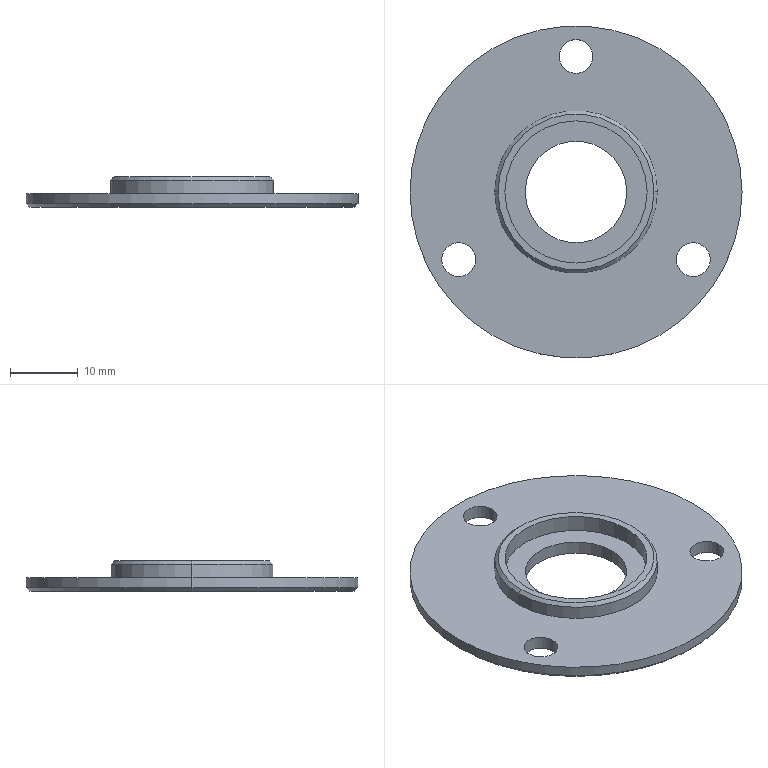Part | SolidWorks | features ICE 4, Chamfer 1, Extrusion 1 | 1 solid | 22 faces | box 49 x 49 x 4.5 mm | volume 3537 mm3 | cylinder 14 | cone 4 | plane 4 | commonest cylinder face diameters 5 x6 15 x2 21 x2 24 x2 49 x2
STEP:
#1=CARTESIAN_POINT('',(11.5,0.,4.5));
#2=VERTEX_POINT('',#1);
#3=CARTESIAN_POINT('',(-11.5,0.,4.5));
#4=VERTEX_POINT('',#3);
#5=CARTESIAN_POINT('',(0.,0.,4.5));
#6=DIRECTION('',(0.,0.,1.));
#7=DIRECTION('',(1.,0.,0.));
#8=AXIS2_PLACEMENT_3D('',#5,#6,#7);
#9=CIRCLE('',#8,11.5);
#10=EDGE_CURVE('',#2,#4,#9,.T.);
#11=ORIENTED_EDGE('',*,*,#10,.F.);
#12=CARTESIAN_POINT('',(12.,0.,4.));
#13=VERTEX_POINT('',#12);
#14=CARTESIAN_POINT('',(11.5,0.,4.5));
#15=DIRECTION('',(0.7071,0.,-0.7071));
#16=VECTOR('',#15,1000.);
#17=LINE('',#14,#16);
#18=EDGE_CURVE('',#2,#13,#17,.T.);
#19=ORIENTED_EDGE('',*,*,#18,.T.);
#20=CARTESIAN_POINT('',(-12.,0.,4.));
#21=VERTEX_POINT('',#20);
#22=CARTESIAN_POINT('',(0.,0.,4.));
#23=DIRECTION('',(0.,0.,-1.));
#24=DIRECTION('',(1.,0.,0.));
#25=AXIS2_PLACEMENT_3D('',#22,#23,#24);
#26=CIRCLE('',#25,12.);
#27=EDGE_CURVE('',#21,#13,#26,.T.);
#28=ORIENTED_EDGE('',*,*,#27,.F.);
#29=CARTESIAN_POINT('',(-11.5,0.,4.5));
#30=DIRECTION('',(-0.7071,0.,-0.7071));
#31=VECTOR('',#30,1000.);
#32=LINE('',#29,#31);
#33=EDGE_CURVE('',#4,#21,#32,.T.);
#34=ORIENTED_EDGE('',*,*,#33,.F.);
#35=EDGE_LOOP('',(#11,#19,#28,#34));
#36=FACE_OUTER_BOUND('',#35,.T.);
#37=CARTESIAN_POINT('',(0.,0.,4.5));
#38=DIRECTION('',(0.,0.,-1.));
#39=DIRECTION('',(-1.,0.,0.));
#40=AXIS2_PLACEMENT_3D('',#37,#38,#39);
#41=CONICAL_SURFACE('',#40,11.5,0.7854);
#42=ADVANCED_FACE('',(#36),#41,.T.);
#43=CARTESIAN_POINT('',(-24.,0.,0.));
#44=VERTEX_POINT('',#43);
#45=CARTESIAN_POINT('',(24.,0.,0.));
#46=VERTEX_POINT('',#45);
#47=CARTESIAN_POINT('',(0.,0.,0.));
#48=DIRECTION('',(0.,0.,-1.));
#49=DIRECTION('',(1.,0.,0.));
#50=AXIS2_PLACEMENT_3D('',#47,#48,#49);
#51=CIRCLE('',#50,24.);
#52=EDGE_CURVE('',#44,#46,#51,.T.);
#53=ORIENTED_EDGE('',*,*,#52,.F.);
#54=CARTESIAN_POINT('',(-24.5,0.,0.5));
#55=VERTEX_POINT('',#54);
#56=CARTESIAN_POINT('',(-24.5,0.,0.5));
#57=DIRECTION('',(-0.7071,0.,0.7071));
#58=VECTOR('',#57,1000.);
#59=LINE('',#56,#58);
#60=EDGE_CURVE('',#44,#55,#59,.T.);
#61=ORIENTED_EDGE('',*,*,#60,.T.);
#62=CARTESIAN_POINT('',(24.5,0.,0.5));
#63=VERTEX_POINT('',#62);
#64=CARTESIAN_POINT('',(0.,0.,0.5));
#65=DIRECTION('',(0.,0.,1.));
#66=DIRECTION('',(1.,0.,0.));
#67=AXIS2_PLACEMENT_3D('',#64,#65,#66);
#68=CIRCLE('',#67,24.5);
#69=EDGE_CURVE('',#63,#55,#68,.T.);
#70=ORIENTED_EDGE('',*,*,#69,.F.);
#71=CARTESIAN_POINT('',(24.5,0.,0.5));
#72=DIRECTION('',(0.7071,0.,0.7071));
#73=VECTOR('',#72,1000.);
#74=LINE('',#71,#73);
#75=EDGE_CURVE('',#46,#63,#74,.T.);
#76=ORIENTED_EDGE('',*,*,#75,.F.);
#77=EDGE_LOOP('',(#53,#61,#70,#76));
#78=FACE_OUTER_BOUND('',#77,.T.);
#79=CARTESIAN_POINT('',(0.,0.,0.5));
#80=DIRECTION('',(0.,0.,1.));
#81=DIRECTION('',(1.,0.,0.));
#82=AXIS2_PLACEMENT_3D('',#79,#80,#81);
#83=CONICAL_SURFACE('',#82,24.5,0.7854);
#84=ADVANCED_FACE('',(#78),#83,.T.);
#85=CARTESIAN_POINT('',(-2.5,20.,0.));
#86=VERTEX_POINT('',#85);
#87=CARTESIAN_POINT('',(2.5,20.,0.));
#88=VERTEX_POINT('',#87);
#89=CARTESIAN_POINT('',(0.,20.,0.));
#90=DIRECTION('',(0.,0.,1.));
#91=DIRECTION('',(1.,0.,0.));
#92=AXIS2_PLACEMENT_3D('',#89,#90,#91);
#93=CIRCLE('',#92,2.5);
#94=EDGE_CURVE('',#86,#88,#93,.T.);
#95=ORIENTED_EDGE('',*,*,#94,.F.);
#96=CARTESIAN_POINT('',(-2.5,20.,2.));
#97=VERTEX_POINT('',#96);
#98=CARTESIAN_POINT('',(-2.5,20.,-0.5));
#99=DIRECTION('',(0.,0.,1.));
#100=VECTOR('',#99,1000.);
#101=LINE('',#98,#100);
#102=EDGE_CURVE('',#86,#97,#101,.T.);
#103=ORIENTED_EDGE('',*,*,#102,.T.);
#104=CARTESIAN_POINT('',(2.5,20.,2.));
#105=VERTEX_POINT('',#104);
#106=CARTESIAN_POINT('',(0.,20.,2.));
#107=DIRECTION('',(0.,0.,1.));
#108=DIRECTION('',(1.,0.,0.));
#109=AXIS2_PLACEMENT_3D('',#106,#107,#108);
#110=CIRCLE('',#109,2.5);
#111=EDGE_CURVE('',#97,#105,#110,.T.);
#112=ORIENTED_EDGE('',*,*,#111,.T.);
#113=CARTESIAN_POINT('',(2.5,20.,-0.5));
#114=DIRECTION('',(0.,0.,1.));
#115=VECTOR('',#114,1000.);
#116=LINE('',#113,#115);
#117=EDGE_CURVE('',#88,#105,#116,.T.);
#118=ORIENTED_EDGE('',*,*,#117,.F.);
#119=EDGE_LOOP('',(#95,#103,#112,#118));
#120=FACE_OUTER_BOUND('',#119,.T.);
#121=CARTESIAN_POINT('',(0.,20.,-0.5));
#122=DIRECTION('',(0.,0.,1.));
#123=DIRECTION('',(1.,0.,0.));
#124=AXIS2_PLACEMENT_3D('',#121,#122,#123);
#125=CYLINDRICAL_SURFACE('',#124,2.5);
#126=ADVANCED_FACE('',(#120),#125,.F.);
#127=CARTESIAN_POINT('',(14.821,-10.,0.));
#128=VERTEX_POINT('',#127);
#129=CARTESIAN_POINT('',(19.821,-10.,0.));
#130=VERTEX_POINT('',#129);
#131=CARTESIAN_POINT('',(17.321,-10.,0.));
#132=DIRECTION('',(0.,0.,1.));
#133=DIRECTION('',(1.,0.,0.));
#134=AXIS2_PLACEMENT_3D('',#131,#132,#133);
#135=CIRCLE('',#134,2.5);
#136=EDGE_CURVE('',#128,#130,#135,.T.);
#137=ORIENTED_EDGE('',*,*,#136,.F.);
#138=CARTESIAN_POINT('',(14.821,-10.,2.));
#139=VERTEX_POINT('',#138);
#140=CARTESIAN_POINT('',(14.821,-10.,-0.5));
#141=DIRECTION('',(0.,0.,1.));
#142=VECTOR('',#141,1000.);
#143=LINE('',#140,#142);
#144=EDGE_CURVE('',#128,#139,#143,.T.);
#145=ORIENTED_EDGE('',*,*,#144,.T.);
#146=CARTESIAN_POINT('',(19.821,-10.,2.));
#147=VERTEX_POINT('',#146);
#148=CARTESIAN_POINT('',(17.321,-10.,2.));
#149=DIRECTION('',(0.,0.,1.));
#150=DIRECTION('',(1.,0.,0.));
#151=AXIS2_PLACEMENT_3D('',#148,#149,#150);
#152=CIRCLE('',#151,2.5);
#153=EDGE_CURVE('',#139,#147,#152,.T.);
#154=ORIENTED_EDGE('',*,*,#153,.T.);
#155=CARTESIAN_POINT('',(19.821,-10.,-0.5));
#156=DIRECTION('',(0.,0.,1.));
#157=VECTOR('',#156,1000.);
#158=LINE('',#155,#157);
#159=EDGE_CURVE('',#130,#147,#158,.T.);
#160=ORIENTED_EDGE('',*,*,#159,.F.);
#161=EDGE_LOOP('',(#137,#145,#154,#160));
#162=FACE_OUTER_BOUND('',#161,.T.);
#163=CARTESIAN_POINT('',(17.321,-10.,-0.5));
#164=DIRECTION('',(0.,0.,1.));
#165=DIRECTION('',(1.,0.,0.));
#166=AXIS2_PLACEMENT_3D('',#163,#164,#165);
#167=CYLINDRICAL_SURFACE('',#166,2.5);
#168=ADVANCED_FACE('',(#162),#167,.F.);
#169=CARTESIAN_POINT('',(-19.821,-10.,0.));
#170=VERTEX_POINT('',#169);
#171=CARTESIAN_POINT('',(-14.821,-10.,0.));
#172=VERTEX_POINT('',#171);
#173=CARTESIAN_POINT('',(-17.321,-10.,0.));
#174=DIRECTION('',(0.,0.,1.));
#175=DIRECTION('',(1.,0.,0.));
#176=AXIS2_PLACEMENT_3D('',#173,#174,#175);
#177=CIRCLE('',#176,2.5);
#178=EDGE_CURVE('',#170,#172,#177,.T.);
#179=ORIENTED_EDGE('',*,*,#178,.F.);
#180=CARTESIAN_POINT('',(-19.821,-10.,2.));
#181=VERTEX_POINT('',#180);
#182=CARTESIAN_POINT('',(-19.821,-10.,-0.5));
#183=DIRECTION('',(0.,0.,1.));
#184=VECTOR('',#183,1000.);
#185=LINE('',#182,#184);
#186=EDGE_CURVE('',#170,#181,#185,.T.);
#187=ORIENTED_EDGE('',*,*,#186,.T.);
#188=CARTESIAN_POINT('',(-14.821,-10.,2.));
#189=VERTEX_POINT('',#188);
#190=CARTESIAN_POINT('',(-17.321,-10.,2.));
#191=DIRECTION('',(0.,0.,1.));
#192=DIRECTION('',(1.,0.,0.));
#193=AXIS2_PLACEMENT_3D('',#190,#191,#192);
#194=CIRCLE('',#193,2.5);
#195=EDGE_CURVE('',#181,#189,#194,.T.);
#196=ORIENTED_EDGE('',*,*,#195,.T.);
#197=CARTESIAN_POINT('',(-14.821,-10.,-0.5));
#198=DIRECTION('',(0.,0.,1.));
#199=VECTOR('',#198,1000.);
#200=LINE('',#197,#199);
#201=EDGE_CURVE('',#172,#189,#200,.T.);
#202=ORIENTED_EDGE('',*,*,#201,.F.);
#203=EDGE_LOOP('',(#179,#187,#196,#202));
#204=FACE_OUTER_BOUND('',#203,.T.);
#205=CARTESIAN_POINT('',(-17.321,-10.,-0.5));
#206=DIRECTION('',(0.,0.,1.));
#207=DIRECTION('',(1.,0.,0.));
#208=AXIS2_PLACEMENT_3D('',#205,#206,#207);
#209=CYLINDRICAL_SURFACE('',#208,2.5);
#210=ADVANCED_FACE('',(#204),#209,.F.);
#211=CARTESIAN_POINT('',(-7.5,0.,0.));
#212=VERTEX_POINT('',#211);
#213=CARTESIAN_POINT('',(7.5,0.,0.));
#214=VERTEX_POINT('',#213);
#215=CARTESIAN_POINT('',(0.,0.,0.));
#216=DIRECTION('',(0.,0.,1.));
#217=DIRECTION('',(1.,0.,0.));
#218=AXIS2_PLACEMENT_3D('',#215,#216,#217);
#219=CIRCLE('',#218,7.5);
#220=EDGE_CURVE('',#212,#214,#219,.T.);
#221=ORIENTED_EDGE('',*,*,#220,.F.);
#222=CARTESIAN_POINT('',(-7.5,0.,2.));
#223=VERTEX_POINT('',#222);
#224=CARTESIAN_POINT('',(-7.5,0.,-0.5));
#225=DIRECTION('',(0.,0.,1.));
#226=VECTOR('',#225,1000.);
#227=LINE('',#224,#226);
#228=EDGE_CURVE('',#212,#223,#227,.T.);
#229=ORIENTED_EDGE('',*,*,#228,.T.);
#230=CARTESIAN_POINT('',(7.5,0.,2.));
#231=VERTEX_POINT('',#230);
#232=CARTESIAN_POINT('',(0.,0.,2.));
#233=DIRECTION('',(0.,0.,1.));
#234=DIRECTION('',(1.,0.,0.));
#235=AXIS2_PLACEMENT_3D('',#232,#233,#234);
#236=CIRCLE('',#235,7.5);
#237=EDGE_CURVE('',#223,#231,#236,.T.);
#238=ORIENTED_EDGE('',*,*,#237,.T.);
#239=CARTESIAN_POINT('',(7.5,0.,-0.5));
#240=DIRECTION('',(0.,0.,1.));
#241=VECTOR('',#240,1000.);
#242=LINE('',#239,#241);
#243=EDGE_CURVE('',#214,#231,#242,.T.);
#244=ORIENTED_EDGE('',*,*,#243,.F.);
#245=EDGE_LOOP('',(#221,#229,#238,#244));
#246=FACE_OUTER_BOUND('',#245,.T.);
#247=CARTESIAN_POINT('',(0.,0.,-0.5));
#248=DIRECTION('',(0.,0.,1.));
#249=DIRECTION('',(1.,0.,0.));
#250=AXIS2_PLACEMENT_3D('',#247,#248,#249);
#251=CYLINDRICAL_SURFACE('',#250,7.5);
#252=ADVANCED_FACE('',(#246),#251,.F.);
#253=CARTESIAN_POINT('',(-10.5,0.,2.));
#254=VERTEX_POINT('',#253);
#255=CARTESIAN_POINT('',(10.5,0.,2.));
#256=VERTEX_POINT('',#255);
#257=CARTESIAN_POINT('',(0.,0.,2.));
#258=DIRECTION('',(0.,0.,1.));
#259=DIRECTION('',(1.,0.,0.));
#260=AXIS2_PLACEMENT_3D('',#257,#258,#259);
#261=CIRCLE('',#260,10.5);
#262=EDGE_CURVE('',#254,#256,#261,.T.);
#263=ORIENTED_EDGE('',*,*,#262,.F.);
#264=CARTESIAN_POINT('',(-10.5,0.,4.5));
#265=VERTEX_POINT('',#264);
#266=CARTESIAN_POINT('',(-10.5,0.,2.));
#267=DIRECTION('',(0.,0.,1.));
#268=VECTOR('',#267,1000.);
#269=LINE('',#266,#268);
#270=EDGE_CURVE('',#254,#265,#269,.T.);
#271=ORIENTED_EDGE('',*,*,#270,.T.);
#272=CARTESIAN_POINT('',(10.5,0.,4.5));
#273=VERTEX_POINT('',#272);
#274=CARTESIAN_POINT('',(0.,0.,4.5));
#275=DIRECTION('',(0.,0.,1.));
#276=DIRECTION('',(1.,0.,0.));
#277=AXIS2_PLACEMENT_3D('',#274,#275,#276);
#278=CIRCLE('',#277,10.5);
#279=EDGE_CURVE('',#265,#273,#278,.T.);
#280=ORIENTED_EDGE('',*,*,#279,.T.);
#281=CARTESIAN_POINT('',(10.5,0.,2.));
#282=DIRECTION('',(0.,0.,1.));
#283=VECTOR('',#282,1000.);
#284=LINE('',#281,#283);
#285=EDGE_CURVE('',#256,#273,#284,.T.);
#286=ORIENTED_EDGE('',*,*,#285,.F.);
#287=EDGE_LOOP('',(#263,#271,#280,#286));
#288=FACE_OUTER_BOUND('',#287,.T.);
#289=CARTESIAN_POINT('',(0.,0.,2.));
#290=DIRECTION('',(0.,0.,1.));
#291=DIRECTION('',(1.,0.,0.));
#292=AXIS2_PLACEMENT_3D('',#289,#290,#291);
#293=CYLINDRICAL_SURFACE('',#292,10.5);
#294=ADVANCED_FACE('',(#288),#293,.F.);
#295=ORIENTED_EDGE('',*,*,#27,.T.);
#296=CARTESIAN_POINT('',(12.,0.,2.));
#297=VERTEX_POINT('',#296);
#298=CARTESIAN_POINT('',(12.,0.,4.5));
#299=DIRECTION('',(0.,0.,-1.));
#300=VECTOR('',#299,1000.);
#301=LINE('',#298,#300);
#302=EDGE_CURVE('',#13,#297,#301,.T.);
#303=ORIENTED_EDGE('',*,*,#302,.T.);
#304=CARTESIAN_POINT('',(-12.,0.,2.));
#305=VERTEX_POINT('',#304);
#306=CARTESIAN_POINT('',(0.,0.,2.));
#307=DIRECTION('',(0.,0.,1.));
#308=DIRECTION('',(1.,0.,0.));
#309=AXIS2_PLACEMENT_3D('',#306,#307,#308);
#310=CIRCLE('',#309,12.);
#311=EDGE_CURVE('',#297,#305,#310,.T.);
#312=ORIENTED_EDGE('',*,*,#311,.T.);
#313=CARTESIAN_POINT('',(-12.,0.,4.5));
#314=DIRECTION('',(0.,0.,-1.));
#315=VECTOR('',#314,1000.);
#316=LINE('',#313,#315);
#317=EDGE_CURVE('',#21,#305,#316,.T.);
#318=ORIENTED_EDGE('',*,*,#317,.F.);
#319=EDGE_LOOP('',(#295,#303,#312,#318));
#320=FACE_OUTER_BOUND('',#319,.T.);
#321=CARTESIAN_POINT('',(0.,0.,4.5));
#322=DIRECTION('',(0.,0.,-1.));
#323=DIRECTION('',(-1.,0.,0.));
#324=AXIS2_PLACEMENT_3D('',#321,#322,#323);
#325=CYLINDRICAL_SURFACE('',#324,12.);
#326=ADVANCED_FACE('',(#320),#325,.T.);
#327=CARTESIAN_POINT('',(24.5,0.,2.));
#328=VERTEX_POINT('',#327);
#329=CARTESIAN_POINT('',(-24.5,0.,2.));
#330=VERTEX_POINT('',#329);
#331=CARTESIAN_POINT('',(0.,0.,2.));
#332=DIRECTION('',(0.,0.,1.));
#333=DIRECTION('',(1.,0.,0.));
#334=AXIS2_PLACEMENT_3D('',#331,#332,#333);
#335=CIRCLE('',#334,24.5);
#336=EDGE_CURVE('',#328,#330,#335,.T.);
#337=ORIENTED_EDGE('',*,*,#336,.F.);
#338=CARTESIAN_POINT('',(24.5,0.,2.));
#339=DIRECTION('',(0.,0.,-1.));
#340=VECTOR('',#339,1000.);
#341=LINE('',#338,#340);
#342=EDGE_CURVE('',#328,#63,#341,.T.);
#343=ORIENTED_EDGE('',*,*,#342,.T.);
#344=ORIENTED_EDGE('',*,*,#69,.T.);
#345=CARTESIAN_POINT('',(-24.5,0.,2.));
#346=DIRECTION('',(0.,0.,-1.));
#347=VECTOR('',#346,1000.);
#348=LINE('',#345,#347);
#349=EDGE_CURVE('',#330,#55,#348,.T.);
#350=ORIENTED_EDGE('',*,*,#349,.F.);
#351=EDGE_LOOP('',(#337,#343,#344,#350));
#352=FACE_OUTER_BOUND('',#351,.T.);
#353=CARTESIAN_POINT('',(0.,0.,2.));
#354=DIRECTION('',(0.,0.,-1.));
#355=DIRECTION('',(-1.,0.,0.));
#356=AXIS2_PLACEMENT_3D('',#353,#354,#355);
#357=CYLINDRICAL_SURFACE('',#356,24.5);
#358=ADVANCED_FACE('',(#352),#357,.T.);
#359=ORIENTED_EDGE('',*,*,#342,.F.);
#360=CARTESIAN_POINT('',(0.,0.,2.));
#361=DIRECTION('',(0.,0.,1.));
#362=DIRECTION('',(1.,0.,0.));
#363=AXIS2_PLACEMENT_3D('',#360,#361,#362);
#364=CIRCLE('',#363,24.5);
#365=EDGE_CURVE('',#330,#328,#364,.T.);
#366=ORIENTED_EDGE('',*,*,#365,.F.);
#367=ORIENTED_EDGE('',*,*,#349,.T.);
#368=CARTESIAN_POINT('',(0.,0.,0.5));
#369=DIRECTION('',(0.,0.,1.));
#370=DIRECTION('',(1.,0.,0.));
#371=AXIS2_PLACEMENT_3D('',#368,#369,#370);
#372=CIRCLE('',#371,24.5);
#373=EDGE_CURVE('',#55,#63,#372,.T.);
#374=ORIENTED_EDGE('',*,*,#373,.T.);
#375=EDGE_LOOP('',(#359,#366,#367,#374));
#376=FACE_OUTER_BOUND('',#375,.T.);
#377=CARTESIAN_POINT('',(0.,0.,2.));
#378=DIRECTION('',(0.,0.,-1.));
#379=DIRECTION('',(-1.,0.,0.));
#380=AXIS2_PLACEMENT_3D('',#377,#378,#379);
#381=CYLINDRICAL_SURFACE('',#380,24.5);
#382=ADVANCED_FACE('',(#376),#381,.T.);
#383=CARTESIAN_POINT('',(0.,20.,2.));
#384=DIRECTION('',(0.,0.,1.));
#385=DIRECTION('',(1.,0.,0.));
#386=AXIS2_PLACEMENT_3D('',#383,#384,#385);
#387=CIRCLE('',#386,2.5);
#388=EDGE_CURVE('',#105,#97,#387,.T.);
#389=ORIENTED_EDGE('',*,*,#388,.F.);
#390=ORIENTED_EDGE('',*,*,#111,.F.);
#391=EDGE_LOOP('',(#389,#390));
#392=FACE_BOUND('',#391,.T.);
#393=CARTESIAN_POINT('',(17.321,-10.,2.));
#394=DIRECTION('',(0.,0.,1.));
#395=DIRECTION('',(1.,0.,0.));
#396=AXIS2_PLACEMENT_3D('',#393,#394,#395);
#397=CIRCLE('',#396,2.5);
#398=EDGE_CURVE('',#147,#139,#397,.T.);
#399=ORIENTED_EDGE('',*,*,#398,.F.);
#400=ORIENTED_EDGE('',*,*,#153,.F.);
#401=EDGE_LOOP('',(#399,#400));
#402=FACE_BOUND('',#401,.T.);
#403=CARTESIAN_POINT('',(-17.321,-10.,2.));
#404=DIRECTION('',(0.,0.,1.));
#405=DIRECTION('',(1.,0.,0.));
#406=AXIS2_PLACEMENT_3D('',#403,#404,#405);
#407=CIRCLE('',#406,2.5);
#408=EDGE_CURVE('',#189,#181,#407,.T.);
#409=ORIENTED_EDGE('',*,*,#408,.F.);
#410=ORIENTED_EDGE('',*,*,#195,.F.);
#411=EDGE_LOOP('',(#409,#410));
#412=FACE_BOUND('',#411,.T.);
#413=CARTESIAN_POINT('',(0.,0.,2.));
#414=DIRECTION('',(0.,0.,1.));
#415=DIRECTION('',(1.,0.,0.));
#416=AXIS2_PLACEMENT_3D('',#413,#414,#415);
#417=CIRCLE('',#416,12.);
#418=EDGE_CURVE('',#305,#297,#417,.T.);
#419=ORIENTED_EDGE('',*,*,#418,.F.);
#420=ORIENTED_EDGE('',*,*,#311,.F.);
#421=EDGE_LOOP('',(#419,#420));
#422=FACE_BOUND('',#421,.T.);
#423=ORIENTED_EDGE('',*,*,#365,.T.);
#424=ORIENTED_EDGE('',*,*,#336,.T.);
#425=EDGE_LOOP('',(#423,#424));
#426=FACE_OUTER_BOUND('',#425,.T.);
#427=CARTESIAN_POINT('',(0.,0.,2.));
#428=DIRECTION('',(0.,0.,1.));
#429=DIRECTION('',(1.,0.,0.));
#430=AXIS2_PLACEMENT_3D('',#427,#428,#429);
#431=PLANE('',#430);
#432=ADVANCED_FACE('',(#392,#402,#412,#422,#426),#431,.T.);
#433=CARTESIAN_POINT('',(0.,0.,0.));
#434=DIRECTION('',(0.,0.,-1.));
#435=DIRECTION('',(1.,0.,0.));
#436=AXIS2_PLACEMENT_3D('',#433,#434,#435);
#437=CIRCLE('',#436,24.);
#438=EDGE_CURVE('',#46,#44,#437,.T.);
#439=ORIENTED_EDGE('',*,*,#438,.T.);
#440=ORIENTED_EDGE('',*,*,#52,.T.);
#441=EDGE_LOOP('',(#439,#440));
#442=FACE_OUTER_BOUND('',#441,.T.);
#443=CARTESIAN_POINT('',(0.,20.,0.));
#444=DIRECTION('',(0.,0.,1.));
#445=DIRECTION('',(1.,0.,0.));
#446=AXIS2_PLACEMENT_3D('',#443,#444,#445);
#447=CIRCLE('',#446,2.5);
#448=EDGE_CURVE('',#88,#86,#447,.T.);
#449=ORIENTED_EDGE('',*,*,#448,.T.);
#450=ORIENTED_EDGE('',*,*,#94,.T.);
#451=EDGE_LOOP('',(#449,#450));
#452=FACE_BOUND('',#451,.T.);
#453=CARTESIAN_POINT('',(17.321,-10.,0.));
#454=DIRECTION('',(0.,0.,1.));
#455=DIRECTION('',(1.,0.,0.));
#456=AXIS2_PLACEMENT_3D('',#453,#454,#455);
#457=CIRCLE('',#456,2.5);
#458=EDGE_CURVE('',#130,#128,#457,.T.);
#459=ORIENTED_EDGE('',*,*,#458,.T.);
#460=ORIENTED_EDGE('',*,*,#136,.T.);
#461=EDGE_LOOP('',(#459,#460));
#462=FACE_BOUND('',#461,.T.);
#463=CARTESIAN_POINT('',(-17.321,-10.,0.));
#464=DIRECTION('',(0.,0.,1.));
#465=DIRECTION('',(1.,0.,0.));
#466=AXIS2_PLACEMENT_3D('',#463,#464,#465);
#467=CIRCLE('',#466,2.5);
#468=EDGE_CURVE('',#172,#170,#467,.T.);
#469=ORIENTED_EDGE('',*,*,#468,.T.);
#470=ORIENTED_EDGE('',*,*,#178,.T.);
#471=EDGE_LOOP('',(#469,#470));
#472=FACE_BOUND('',#471,.T.);
#473=CARTESIAN_POINT('',(0.,0.,0.));
#474=DIRECTION('',(0.,0.,1.));
#475=DIRECTION('',(1.,0.,0.));
#476=AXIS2_PLACEMENT_3D('',#473,#474,#475);
#477=CIRCLE('',#476,7.5);
#478=EDGE_CURVE('',#214,#212,#477,.T.);
#479=ORIENTED_EDGE('',*,*,#478,.T.);
#480=ORIENTED_EDGE('',*,*,#220,.T.);
#481=EDGE_LOOP('',(#479,#480));
#482=FACE_BOUND('',#481,.T.);
#483=CARTESIAN_POINT('',(0.,0.,0.));
#484=DIRECTION('',(0.,0.,1.));
#485=DIRECTION('',(1.,0.,0.));
#486=AXIS2_PLACEMENT_3D('',#483,#484,#485);
#487=PLANE('',#486);
#488=ADVANCED_FACE('',(#442,#452,#462,#472,#482),#487,.F.);
#489=ORIENTED_EDGE('',*,*,#302,.F.);
#490=CARTESIAN_POINT('',(0.,0.,4.));
#491=DIRECTION('',(0.,0.,-1.));
#492=DIRECTION('',(1.,0.,0.));
#493=AXIS2_PLACEMENT_3D('',#490,#491,#492);
#494=CIRCLE('',#493,12.);
#495=EDGE_CURVE('',#13,#21,#494,.T.);
#496=ORIENTED_EDGE('',*,*,#495,.T.);
#497=ORIENTED_EDGE('',*,*,#317,.T.);
#498=ORIENTED_EDGE('',*,*,#418,.T.);
#499=EDGE_LOOP('',(#489,#496,#497,#498));
#500=FACE_OUTER_BOUND('',#499,.T.);
#501=CARTESIAN_POINT('',(0.,0.,4.5));
#502=DIRECTION('',(0.,0.,-1.));
#503=DIRECTION('',(-1.,0.,0.));
#504=AXIS2_PLACEMENT_3D('',#501,#502,#503);
#505=CYLINDRICAL_SURFACE('',#504,12.);
#506=ADVANCED_FACE('',(#500),#505,.T.);
#507=CARTESIAN_POINT('',(0.,0.,4.5));
#508=DIRECTION('',(0.,0.,1.));
#509=DIRECTION('',(1.,0.,0.));
#510=AXIS2_PLACEMENT_3D('',#507,#508,#509);
#511=CIRCLE('',#510,11.5);
#512=EDGE_CURVE('',#4,#2,#511,.T.);
#513=ORIENTED_EDGE('',*,*,#512,.T.);
#514=ORIENTED_EDGE('',*,*,#10,.T.);
#515=EDGE_LOOP('',(#513,#514));
#516=FACE_OUTER_BOUND('',#515,.T.);
#517=CARTESIAN_POINT('',(0.,0.,4.5));
#518=DIRECTION('',(0.,0.,1.));
#519=DIRECTION('',(1.,0.,0.));
#520=AXIS2_PLACEMENT_3D('',#517,#518,#519);
#521=CIRCLE('',#520,10.5);
#522=EDGE_CURVE('',#273,#265,#521,.T.);
#523=ORIENTED_EDGE('',*,*,#522,.F.);
#524=ORIENTED_EDGE('',*,*,#279,.F.);
#525=EDGE_LOOP('',(#523,#524));
#526=FACE_BOUND('',#525,.T.);
#527=CARTESIAN_POINT('',(0.,0.,4.5));
#528=DIRECTION('',(0.,0.,1.));
#529=DIRECTION('',(1.,0.,0.));
#530=AXIS2_PLACEMENT_3D('',#527,#528,#529);
#531=PLANE('',#530);
#532=ADVANCED_FACE('',(#516,#526),#531,.T.);
#533=ORIENTED_EDGE('',*,*,#270,.F.);
#534=CARTESIAN_POINT('',(0.,0.,2.));
#535=DIRECTION('',(0.,0.,1.));
#536=DIRECTION('',(1.,0.,0.));
#537=AXIS2_PLACEMENT_3D('',#534,#535,#536);
#538=CIRCLE('',#537,10.5);
#539=EDGE_CURVE('',#256,#254,#538,.T.);
#540=ORIENTED_EDGE('',*,*,#539,.F.);
#541=ORIENTED_EDGE('',*,*,#285,.T.);
#542=ORIENTED_EDGE('',*,*,#522,.T.);
#543=EDGE_LOOP('',(#533,#540,#541,#542));
#544=FACE_OUTER_BOUND('',#543,.T.);
#545=CARTESIAN_POINT('',(0.,0.,2.));
#546=DIRECTION('',(0.,0.,1.));
#547=DIRECTION('',(1.,0.,0.));
#548=AXIS2_PLACEMENT_3D('',#545,#546,#547);
#549=CYLINDRICAL_SURFACE('',#548,10.5);
#550=ADVANCED_FACE('',(#544),#549,.F.);
#551=CARTESIAN_POINT('',(0.,0.,2.));
#552=DIRECTION('',(0.,0.,1.));
#553=DIRECTION('',(1.,0.,0.));
#554=AXIS2_PLACEMENT_3D('',#551,#552,#553);
#555=CIRCLE('',#554,7.5);
#556=EDGE_CURVE('',#231,#223,#555,.T.);
#557=ORIENTED_EDGE('',*,*,#556,.F.);
#558=ORIENTED_EDGE('',*,*,#237,.F.);
#559=EDGE_LOOP('',(#557,#558));
#560=FACE_BOUND('',#559,.T.);
#561=ORIENTED_EDGE('',*,*,#539,.T.);
#562=ORIENTED_EDGE('',*,*,#262,.T.);
#563=EDGE_LOOP('',(#561,#562));
#564=FACE_OUTER_BOUND('',#563,.T.);
#565=CARTESIAN_POINT('',(0.,0.,2.));
#566=DIRECTION('',(0.,0.,1.));
#567=DIRECTION('',(1.,0.,0.));
#568=AXIS2_PLACEMENT_3D('',#565,#566,#567);
#569=PLANE('',#568);
#570=ADVANCED_FACE('',(#560,#564),#569,.T.);
#571=ORIENTED_EDGE('',*,*,#228,.F.);
#572=ORIENTED_EDGE('',*,*,#478,.F.);
#573=ORIENTED_EDGE('',*,*,#243,.T.);
#574=ORIENTED_EDGE('',*,*,#556,.T.);
#575=EDGE_LOOP('',(#571,#572,#573,#574));
#576=FACE_OUTER_BOUND('',#575,.T.);
#577=CARTESIAN_POINT('',(0.,0.,-0.5));
#578=DIRECTION('',(0.,0.,1.));
#579=DIRECTION('',(1.,0.,0.));
#580=AXIS2_PLACEMENT_3D('',#577,#578,#579);
#581=CYLINDRICAL_SURFACE('',#580,7.5);
#582=ADVANCED_FACE('',(#576),#581,.F.);
#583=ORIENTED_EDGE('',*,*,#186,.F.);
#584=ORIENTED_EDGE('',*,*,#468,.F.);
#585=ORIENTED_EDGE('',*,*,#201,.T.);
#586=ORIENTED_EDGE('',*,*,#408,.T.);
#587=EDGE_LOOP('',(#583,#584,#585,#586));
#588=FACE_OUTER_BOUND('',#587,.T.);
#589=CARTESIAN_POINT('',(-17.321,-10.,-0.5));
#590=DIRECTION('',(0.,0.,1.));
#591=DIRECTION('',(1.,0.,0.));
#592=AXIS2_PLACEMENT_3D('',#589,#590,#591);
#593=CYLINDRICAL_SURFACE('',#592,2.5);
#594=ADVANCED_FACE('',(#588),#593,.F.);
#595=ORIENTED_EDGE('',*,*,#144,.F.);
#596=ORIENTED_EDGE('',*,*,#458,.F.);
#597=ORIENTED_EDGE('',*,*,#159,.T.);
#598=ORIENTED_EDGE('',*,*,#398,.T.);
#599=EDGE_LOOP('',(#595,#596,#597,#598));
#600=FACE_OUTER_BOUND('',#599,.T.);
#601=CARTESIAN_POINT('',(17.321,-10.,-0.5));
#602=DIRECTION('',(0.,0.,1.));
#603=DIRECTION('',(1.,0.,0.));
#604=AXIS2_PLACEMENT_3D('',#601,#602,#603);
#605=CYLINDRICAL_SURFACE('',#604,2.5);
#606=ADVANCED_FACE('',(#600),#605,.F.);
#607=ORIENTED_EDGE('',*,*,#102,.F.);
#608=ORIENTED_EDGE('',*,*,#448,.F.);
#609=ORIENTED_EDGE('',*,*,#117,.T.);
#610=ORIENTED_EDGE('',*,*,#388,.T.);
#611=EDGE_LOOP('',(#607,#608,#609,#610));
#612=FACE_OUTER_BOUND('',#611,.T.);
#613=CARTESIAN_POINT('',(0.,20.,-0.5));
#614=DIRECTION('',(0.,0.,1.));
#615=DIRECTION('',(1.,0.,0.));
#616=AXIS2_PLACEMENT_3D('',#613,#614,#615);
#617=CYLINDRICAL_SURFACE('',#616,2.5);
#618=ADVANCED_FACE('',(#612),#617,.F.);
#619=ORIENTED_EDGE('',*,*,#60,.F.);
#620=ORIENTED_EDGE('',*,*,#438,.F.);
#621=ORIENTED_EDGE('',*,*,#75,.T.);
#622=ORIENTED_EDGE('',*,*,#373,.F.);
#623=EDGE_LOOP('',(#619,#620,#621,#622));
#624=FACE_OUTER_BOUND('',#623,.T.);
#625=CARTESIAN_POINT('',(0.,0.,0.5));
#626=DIRECTION('',(0.,0.,1.));
#627=DIRECTION('',(1.,0.,0.));
#628=AXIS2_PLACEMENT_3D('',#625,#626,#627);
#629=CONICAL_SURFACE('',#628,24.5,0.7854);
#630=ADVANCED_FACE('',(#624),#629,.T.);
#631=ORIENTED_EDGE('',*,*,#18,.F.);
#632=ORIENTED_EDGE('',*,*,#512,.F.);
#633=ORIENTED_EDGE('',*,*,#33,.T.);
#634=ORIENTED_EDGE('',*,*,#495,.F.);
#635=EDGE_LOOP('',(#631,#632,#633,#634));
#636=FACE_OUTER_BOUND('',#635,.T.);
#637=CARTESIAN_POINT('',(0.,0.,4.5));
#638=DIRECTION('',(0.,0.,-1.));
#639=DIRECTION('',(-1.,0.,0.));
#640=AXIS2_PLACEMENT_3D('',#637,#638,#639);
#641=CONICAL_SURFACE('',#640,11.5,0.7854);
#642=ADVANCED_FACE('',(#636),#641,.T.);
#643=CLOSED_SHELL('',(#42,#84,#126,#168,#210,#252,#294,#326,#358,#382,#432,#488,#506,#532,#550,#570,#582,#594,#606,#618,#630,#642));
#644=MANIFOLD_SOLID_BREP('',#643);
#645=CARTESIAN_POINT('',(0.,0.,0.));
#646=DIRECTION('',(0.,0.,1.));
#647=DIRECTION('',(1.,0.,0.));
#648=AXIS2_PLACEMENT_3D('',#645,#646,#647);
#649=(LENGTH_UNIT()NAMED_UNIT(*)SI_UNIT(.MILLI.,.METRE.));
#650=UNCERTAINTY_MEASURE_WITH_UNIT(LENGTH_MEASURE(0.00001),#649,'','');
#651=(NAMED_UNIT(*)PLANE_ANGLE_UNIT()SI_UNIT($,.RADIAN.));
#652=(NAMED_UNIT(*)SI_UNIT($,.STERADIAN.)SOLID_ANGLE_UNIT());
#653=(GEOMETRIC_REPRESENTATION_CONTEXT(3)GLOBAL_UNCERTAINTY_ASSIGNED_CONTEXT((#650))GLOBAL_UNIT_ASSIGNED_CONTEXT((#649,#651,#652))REPRESENTATION_CONTEXT('',''));
#654=ADVANCED_BREP_SHAPE_REPRESENTATION('',(#644,#648),#653);